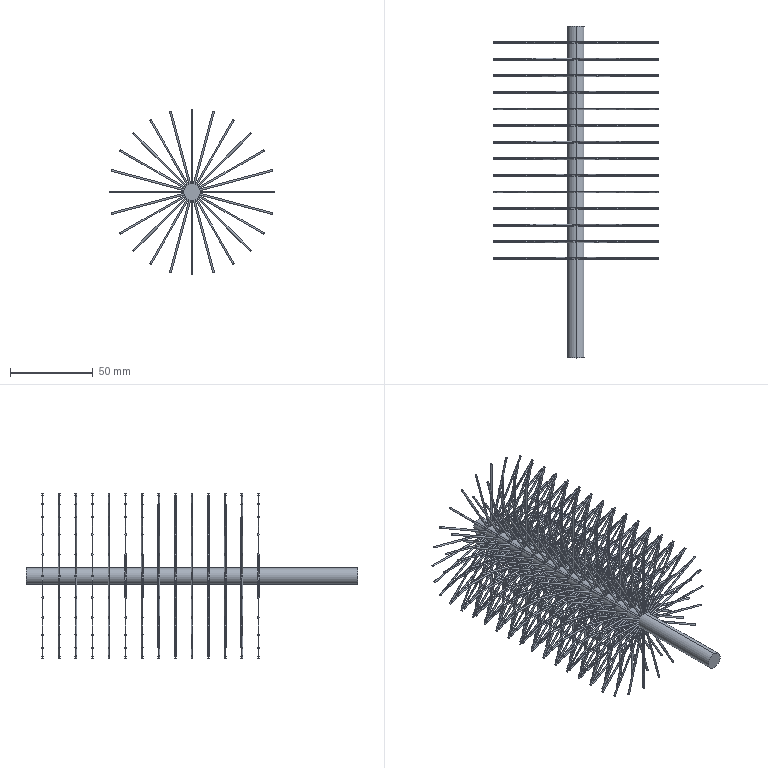Part | SolidWorks | features CirPattern 1, Extrusion 1, ICE 1, LPattern 1, RefAxis 1 | 337 solids | 1348 faces | box 100 x 200 x 100 mm | volume 28903 mm3 | cylinder 674 | plane 674 | commonest cylinder face diameters 1 x672 10 x2